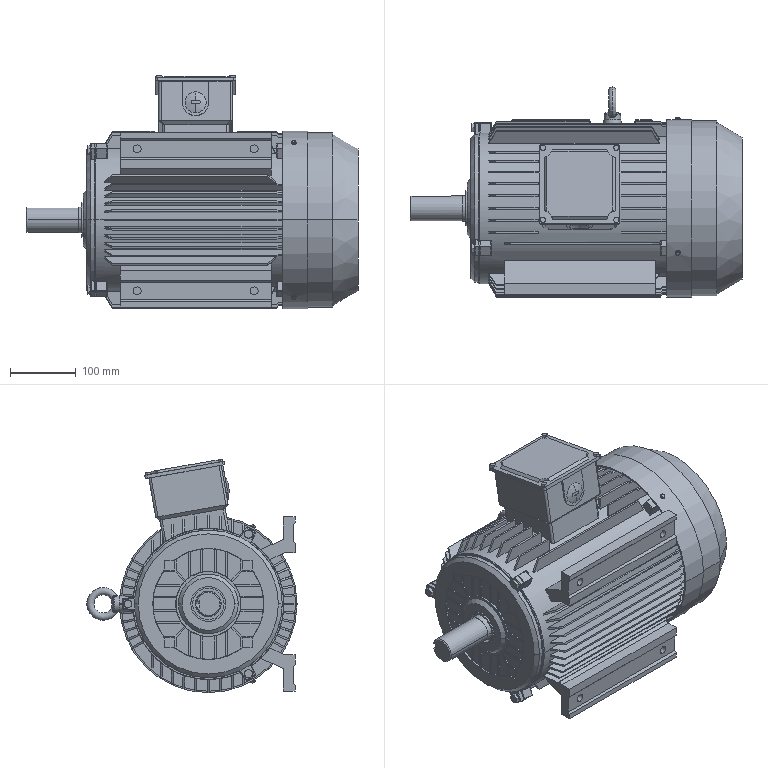Part | SolidWorks | features ICE 21, CirPattern 7, LibraryFeature 7, Extrusion 6, Fillet 6, RevCut 6, Revolution 5, Chamfer 4, CombineBodies 3, MoveCopyBody 3, CurvePattern 2, DeleteBody 2, MirrorSolid 2, CutThin 1, RevCutThin 1 | 1 solid | 876 faces | box 505 x 319.8 x 355 mm | volume 20440913 mm3 | plane 589 | cylinder 140 | cone 97 | sphere 38 | spline 8 | torus 4 | commonest cylinder face diameters 2 x69 6.701 x12 12 x8 7.56 x6 168.683 x6 9.382 x4